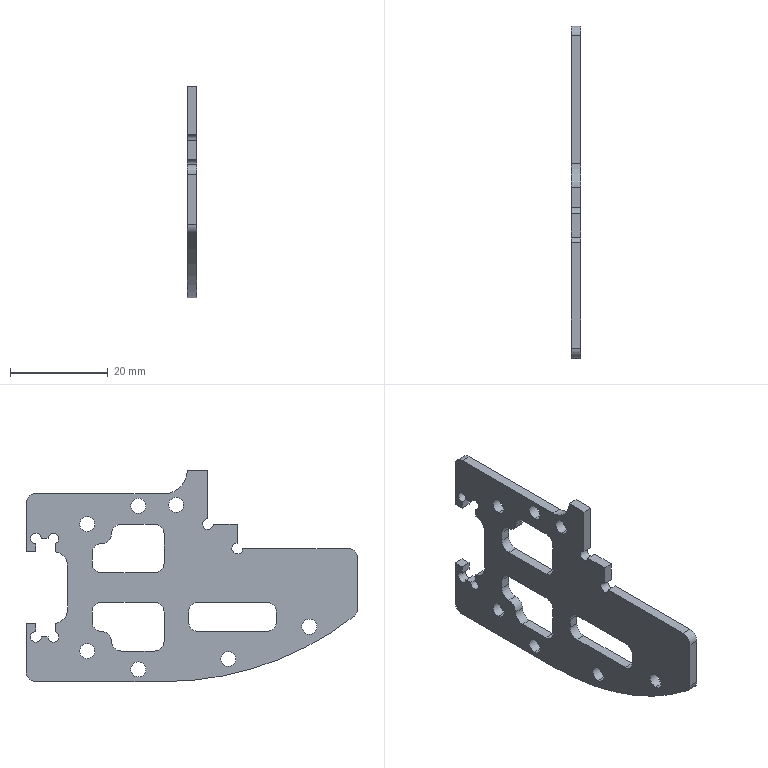Part | SolidWorks | features Fillet 2, Extrusion 1 | 1 solid | 79 faces | box 2 x 67.95 x 43.25 mm | volume 3148 mm3 | cylinder 46 | plane 33 | commonest cylinder face diameters 4 x20 3.1 x14 2.2 x8 6 x2 9.5 x1 126.5 x1